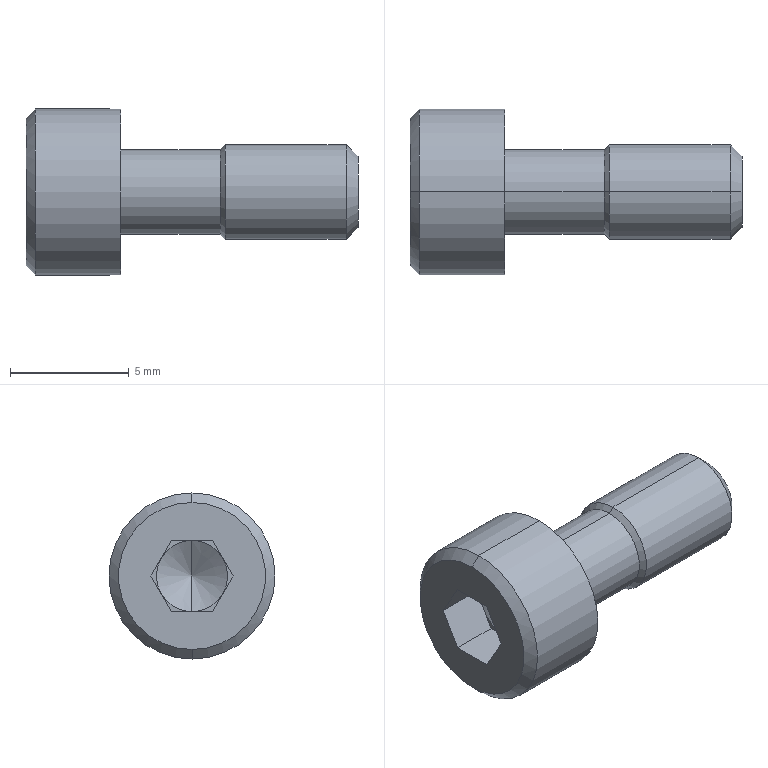Part | STEP file | 0245_Z_030_SCBS4-10_1 | 1 solid | 29 faces | box 14 x 7 x 7 mm | volume 247.861 mm3 | plane 15 | cone 8 | cylinder 6 | commonest cylinder face diameters 3.57 x2 4 x2 7 x2